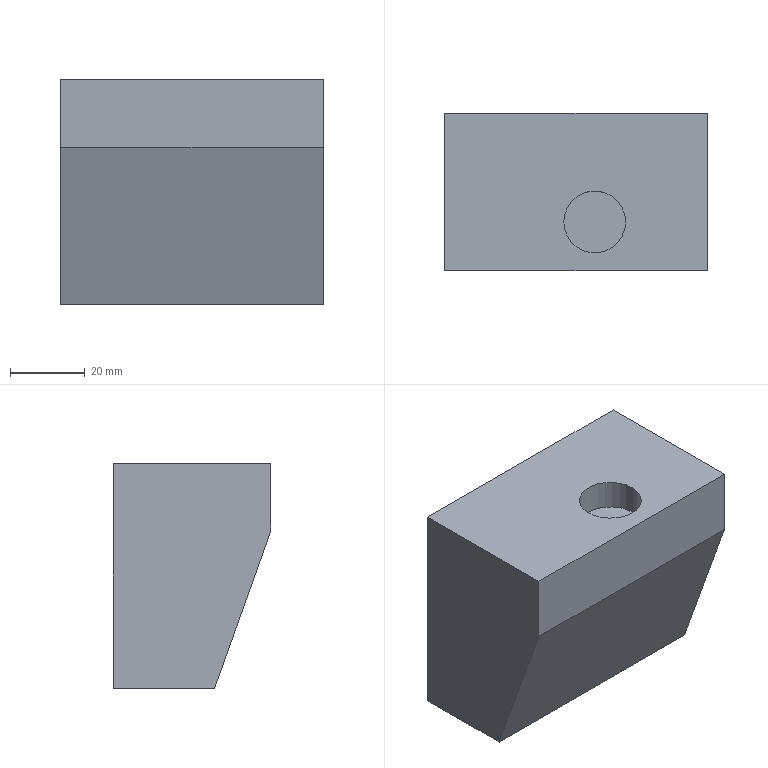Part | SolidWorks | features ICE 2, Extrusion 1 | 1 solid | 10 faces | box 70 x 42 x 60 mm | volume 152639 mm3 | plane 8 | cylinder 2 | commonest cylinder face diameters 16.5 x2
STEP:
#1=CARTESIAN_POINT('',(-8.25,-9.,22.));
#2=VERTEX_POINT('',#1);
#3=CARTESIAN_POINT('',(8.25,-9.,22.));
#4=VERTEX_POINT('',#3);
#5=CARTESIAN_POINT('',(0.,-9.,22.));
#6=DIRECTION('',(0.,0.,1.));
#7=DIRECTION('',(1.,0.,0.));
#8=AXIS2_PLACEMENT_3D('',#5,#6,#7);
#9=CIRCLE('',#8,8.25);
#10=EDGE_CURVE('',#2,#4,#9,.T.);
#11=ORIENTED_EDGE('',*,*,#10,.F.);
#12=CARTESIAN_POINT('',(-8.25,-9.,30.));
#13=VERTEX_POINT('',#12);
#14=CARTESIAN_POINT('',(-8.25,-9.,22.));
#15=DIRECTION('',(0.,0.,1.));
#16=VECTOR('',#15,1000.);
#17=LINE('',#14,#16);
#18=EDGE_CURVE('',#2,#13,#17,.T.);
#19=ORIENTED_EDGE('',*,*,#18,.T.);
#20=CARTESIAN_POINT('',(8.25,-9.,30.));
#21=VERTEX_POINT('',#20);
#22=CARTESIAN_POINT('',(0.,-9.,30.));
#23=DIRECTION('',(0.,0.,1.));
#24=DIRECTION('',(1.,0.,0.));
#25=AXIS2_PLACEMENT_3D('',#22,#23,#24);
#26=CIRCLE('',#25,8.25);
#27=EDGE_CURVE('',#13,#21,#26,.T.);
#28=ORIENTED_EDGE('',*,*,#27,.T.);
#29=CARTESIAN_POINT('',(8.25,-9.,22.));
#30=DIRECTION('',(0.,0.,1.));
#31=VECTOR('',#30,1000.);
#32=LINE('',#29,#31);
#33=EDGE_CURVE('',#4,#21,#32,.T.);
#34=ORIENTED_EDGE('',*,*,#33,.F.);
#35=EDGE_LOOP('',(#11,#19,#28,#34));
#36=FACE_OUTER_BOUND('',#35,.T.);
#37=CARTESIAN_POINT('',(0.,-9.,22.));
#38=DIRECTION('',(0.,0.,1.));
#39=DIRECTION('',(1.,0.,0.));
#40=AXIS2_PLACEMENT_3D('',#37,#38,#39);
#41=CYLINDRICAL_SURFACE('',#40,8.25);
#42=ADVANCED_FACE('',(#36),#41,.F.);
#43=CARTESIAN_POINT('',(30.,20.,30.));
#44=VERTEX_POINT('',#43);
#45=CARTESIAN_POINT('',(30.,-22.,30.));
#46=VERTEX_POINT('',#45);
#47=CARTESIAN_POINT('',(30.,20.,30.));
#48=DIRECTION('',(0.,-1.,0.));
#49=VECTOR('',#48,1000.);
#50=LINE('',#47,#49);
#51=EDGE_CURVE('',#44,#46,#50,.T.);
#52=ORIENTED_EDGE('',*,*,#51,.T.);
#53=CARTESIAN_POINT('',(30.,-22.,12.));
#54=VERTEX_POINT('',#53);
#55=CARTESIAN_POINT('',(30.,-22.,12.));
#56=DIRECTION('',(0.,0.,-1.));
#57=VECTOR('',#56,1000.);
#58=LINE('',#55,#57);
#59=EDGE_CURVE('',#46,#54,#58,.T.);
#60=ORIENTED_EDGE('',*,*,#59,.T.);
#61=CARTESIAN_POINT('',(30.,-7.,-30.));
#62=VERTEX_POINT('',#61);
#63=CARTESIAN_POINT('',(30.,-7.,-30.));
#64=DIRECTION('',(0.,0.3363,-0.9417));
#65=VECTOR('',#64,1000.);
#66=LINE('',#63,#65);
#67=EDGE_CURVE('',#54,#62,#66,.T.);
#68=ORIENTED_EDGE('',*,*,#67,.T.);
#69=CARTESIAN_POINT('',(30.,20.,-30.));
#70=VERTEX_POINT('',#69);
#71=CARTESIAN_POINT('',(30.,20.,-30.));
#72=DIRECTION('',(0.,-1.,0.));
#73=VECTOR('',#72,1000.);
#74=LINE('',#71,#73);
#75=EDGE_CURVE('',#70,#62,#74,.T.);
#76=ORIENTED_EDGE('',*,*,#75,.F.);
#77=CARTESIAN_POINT('',(30.,20.,-30.));
#78=DIRECTION('',(0.,0.,-1.));
#79=VECTOR('',#78,1000.);
#80=LINE('',#77,#79);
#81=EDGE_CURVE('',#44,#70,#80,.T.);
#82=ORIENTED_EDGE('',*,*,#81,.F.);
#83=EDGE_LOOP('',(#52,#60,#68,#76,#82));
#84=FACE_OUTER_BOUND('',#83,.T.);
#85=CARTESIAN_POINT('',(30.,20.,-30.));
#86=DIRECTION('',(-1.,0.,0.));
#87=DIRECTION('',(0.,0.,1.));
#88=AXIS2_PLACEMENT_3D('',#85,#86,#87);
#89=PLANE('',#88);
#90=ADVANCED_FACE('',(#84),#89,.F.);
#91=ORIENTED_EDGE('',*,*,#75,.T.);
#92=CARTESIAN_POINT('',(-40.,-7.,-30.));
#93=VERTEX_POINT('',#92);
#94=CARTESIAN_POINT('',(-40.,-7.,-30.));
#95=DIRECTION('',(1.,0.,0.));
#96=VECTOR('',#95,1000.);
#97=LINE('',#94,#96);
#98=EDGE_CURVE('',#93,#62,#97,.T.);
#99=ORIENTED_EDGE('',*,*,#98,.F.);
#100=CARTESIAN_POINT('',(-40.,20.,-30.));
#101=VERTEX_POINT('',#100);
#102=CARTESIAN_POINT('',(-40.,0.,-30.));
#103=DIRECTION('',(0.,1.,0.));
#104=VECTOR('',#103,1000.);
#105=LINE('',#102,#104);
#106=EDGE_CURVE('',#93,#101,#105,.T.);
#107=ORIENTED_EDGE('',*,*,#106,.T.);
#108=CARTESIAN_POINT('',(-30.,20.,-30.));
#109=DIRECTION('',(-1.,0.,0.));
#110=VECTOR('',#109,1000.);
#111=LINE('',#108,#110);
#112=EDGE_CURVE('',#70,#101,#111,.T.);
#113=ORIENTED_EDGE('',*,*,#112,.F.);
#114=EDGE_LOOP('',(#91,#99,#107,#113));
#115=FACE_OUTER_BOUND('',#114,.T.);
#116=CARTESIAN_POINT('',(-30.,20.,-30.));
#117=DIRECTION('',(0.,0.,1.));
#118=DIRECTION('',(1.,0.,0.));
#119=AXIS2_PLACEMENT_3D('',#116,#117,#118);
#120=PLANE('',#119);
#121=ADVANCED_FACE('',(#115),#120,.F.);
#122=CARTESIAN_POINT('',(0.,-9.,30.));
#123=DIRECTION('',(0.,0.,1.));
#124=DIRECTION('',(1.,0.,0.));
#125=AXIS2_PLACEMENT_3D('',#122,#123,#124);
#126=CIRCLE('',#125,8.25);
#127=EDGE_CURVE('',#21,#13,#126,.T.);
#128=ORIENTED_EDGE('',*,*,#127,.F.);
#129=ORIENTED_EDGE('',*,*,#27,.F.);
#130=EDGE_LOOP('',(#128,#129));
#131=FACE_BOUND('',#130,.T.);
#132=CARTESIAN_POINT('',(-40.,20.,30.));
#133=VERTEX_POINT('',#132);
#134=CARTESIAN_POINT('',(-30.,20.,30.));
#135=DIRECTION('',(1.,0.,0.));
#136=VECTOR('',#135,1000.);
#137=LINE('',#134,#136);
#138=EDGE_CURVE('',#133,#44,#137,.T.);
#139=ORIENTED_EDGE('',*,*,#138,.F.);
#140=CARTESIAN_POINT('',(-40.,-22.,30.));
#141=VERTEX_POINT('',#140);
#142=CARTESIAN_POINT('',(-40.,-22.,30.));
#143=DIRECTION('',(0.,-1.,0.));
#144=VECTOR('',#143,1000.);
#145=LINE('',#142,#144);
#146=EDGE_CURVE('',#133,#141,#145,.T.);
#147=ORIENTED_EDGE('',*,*,#146,.T.);
#148=CARTESIAN_POINT('',(-40.,-22.,30.));
#149=DIRECTION('',(1.,0.,0.));
#150=VECTOR('',#149,1000.);
#151=LINE('',#148,#150);
#152=EDGE_CURVE('',#141,#46,#151,.T.);
#153=ORIENTED_EDGE('',*,*,#152,.T.);
#154=ORIENTED_EDGE('',*,*,#51,.F.);
#155=EDGE_LOOP('',(#139,#147,#153,#154));
#156=FACE_OUTER_BOUND('',#155,.T.);
#157=CARTESIAN_POINT('',(-30.,20.,30.));
#158=DIRECTION('',(0.,0.,-1.));
#159=DIRECTION('',(-1.,0.,0.));
#160=AXIS2_PLACEMENT_3D('',#157,#158,#159);
#161=PLANE('',#160);
#162=ADVANCED_FACE('',(#131,#156),#161,.F.);
#163=ORIENTED_EDGE('',*,*,#81,.T.);
#164=ORIENTED_EDGE('',*,*,#112,.T.);
#165=CARTESIAN_POINT('',(-40.,20.,30.));
#166=DIRECTION('',(0.,0.,1.));
#167=VECTOR('',#166,1000.);
#168=LINE('',#165,#167);
#169=EDGE_CURVE('',#101,#133,#168,.T.);
#170=ORIENTED_EDGE('',*,*,#169,.T.);
#171=ORIENTED_EDGE('',*,*,#138,.T.);
#172=EDGE_LOOP('',(#163,#164,#170,#171));
#173=FACE_OUTER_BOUND('',#172,.T.);
#174=CARTESIAN_POINT('',(0.,20.,0.));
#175=DIRECTION('',(0.,1.,0.));
#176=DIRECTION('',(0.,0.,1.));
#177=AXIS2_PLACEMENT_3D('',#174,#175,#176);
#178=PLANE('',#177);
#179=ADVANCED_FACE('',(#173),#178,.T.);
#180=ORIENTED_EDGE('',*,*,#67,.F.);
#181=CARTESIAN_POINT('',(-40.,-22.,12.));
#182=VERTEX_POINT('',#181);
#183=CARTESIAN_POINT('',(-40.,-22.,12.));
#184=DIRECTION('',(1.,0.,0.));
#185=VECTOR('',#184,1000.);
#186=LINE('',#183,#185);
#187=EDGE_CURVE('',#182,#54,#186,.T.);
#188=ORIENTED_EDGE('',*,*,#187,.F.);
#189=CARTESIAN_POINT('',(-40.,-7.,-30.));
#190=DIRECTION('',(0.,0.3363,-0.9417));
#191=VECTOR('',#190,1000.);
#192=LINE('',#189,#191);
#193=EDGE_CURVE('',#182,#93,#192,.T.);
#194=ORIENTED_EDGE('',*,*,#193,.T.);
#195=ORIENTED_EDGE('',*,*,#98,.T.);
#196=EDGE_LOOP('',(#180,#188,#194,#195));
#197=FACE_OUTER_BOUND('',#196,.T.);
#198=CARTESIAN_POINT('',(-40.,-7.,-30.));
#199=DIRECTION('',(0.,-0.9417,-0.3363));
#200=DIRECTION('',(0.,0.3363,-0.9417));
#201=AXIS2_PLACEMENT_3D('',#198,#199,#200);
#202=PLANE('',#201);
#203=ADVANCED_FACE('',(#197),#202,.T.);
#204=ORIENTED_EDGE('',*,*,#59,.F.);
#205=ORIENTED_EDGE('',*,*,#152,.F.);
#206=CARTESIAN_POINT('',(-40.,-22.,12.));
#207=DIRECTION('',(0.,0.,-1.));
#208=VECTOR('',#207,1000.);
#209=LINE('',#206,#208);
#210=EDGE_CURVE('',#141,#182,#209,.T.);
#211=ORIENTED_EDGE('',*,*,#210,.T.);
#212=ORIENTED_EDGE('',*,*,#187,.T.);
#213=EDGE_LOOP('',(#204,#205,#211,#212));
#214=FACE_OUTER_BOUND('',#213,.T.);
#215=CARTESIAN_POINT('',(-40.,-22.,12.));
#216=DIRECTION('',(0.,-1.,0.));
#217=DIRECTION('',(0.,0.,-1.));
#218=AXIS2_PLACEMENT_3D('',#215,#216,#217);
#219=PLANE('',#218);
#220=ADVANCED_FACE('',(#214),#219,.T.);
#221=ORIENTED_EDGE('',*,*,#169,.F.);
#222=ORIENTED_EDGE('',*,*,#106,.F.);
#223=ORIENTED_EDGE('',*,*,#193,.F.);
#224=ORIENTED_EDGE('',*,*,#210,.F.);
#225=ORIENTED_EDGE('',*,*,#146,.F.);
#226=EDGE_LOOP('',(#221,#222,#223,#224,#225));
#227=FACE_OUTER_BOUND('',#226,.T.);
#228=CARTESIAN_POINT('',(-40.,0.,0.));
#229=DIRECTION('',(-1.,0.,0.));
#230=DIRECTION('',(0.,0.,1.));
#231=AXIS2_PLACEMENT_3D('',#228,#229,#230);
#232=PLANE('',#231);
#233=ADVANCED_FACE('',(#227),#232,.T.);
#234=ORIENTED_EDGE('',*,*,#18,.F.);
#235=CARTESIAN_POINT('',(0.,-9.,22.));
#236=DIRECTION('',(0.,0.,1.));
#237=DIRECTION('',(1.,0.,0.));
#238=AXIS2_PLACEMENT_3D('',#235,#236,#237);
#239=CIRCLE('',#238,8.25);
#240=EDGE_CURVE('',#4,#2,#239,.T.);
#241=ORIENTED_EDGE('',*,*,#240,.F.);
#242=ORIENTED_EDGE('',*,*,#33,.T.);
#243=ORIENTED_EDGE('',*,*,#127,.T.);
#244=EDGE_LOOP('',(#234,#241,#242,#243));
#245=FACE_OUTER_BOUND('',#244,.T.);
#246=CARTESIAN_POINT('',(0.,-9.,22.));
#247=DIRECTION('',(0.,0.,1.));
#248=DIRECTION('',(1.,0.,0.));
#249=AXIS2_PLACEMENT_3D('',#246,#247,#248);
#250=CYLINDRICAL_SURFACE('',#249,8.25);
#251=ADVANCED_FACE('',(#245),#250,.F.);
#252=ORIENTED_EDGE('',*,*,#240,.T.);
#253=ORIENTED_EDGE('',*,*,#10,.T.);
#254=EDGE_LOOP('',(#252,#253));
#255=FACE_OUTER_BOUND('',#254,.T.);
#256=CARTESIAN_POINT('',(0.,-9.,22.));
#257=DIRECTION('',(0.,0.,1.));
#258=DIRECTION('',(1.,0.,0.));
#259=AXIS2_PLACEMENT_3D('',#256,#257,#258);
#260=PLANE('',#259);
#261=ADVANCED_FACE('',(#255),#260,.T.);
#262=CLOSED_SHELL('',(#42,#90,#121,#162,#179,#203,#220,#233,#251,#261));
#263=MANIFOLD_SOLID_BREP('',#262);
#264=CARTESIAN_POINT('',(0.,0.,0.));
#265=DIRECTION('',(0.,0.,1.));
#266=DIRECTION('',(1.,0.,0.));
#267=AXIS2_PLACEMENT_3D('',#264,#265,#266);
#268=(LENGTH_UNIT()NAMED_UNIT(*)SI_UNIT(.MILLI.,.METRE.));
#269=UNCERTAINTY_MEASURE_WITH_UNIT(LENGTH_MEASURE(0.00001),#268,'','');
#270=(NAMED_UNIT(*)PLANE_ANGLE_UNIT()SI_UNIT($,.RADIAN.));
#271=(NAMED_UNIT(*)SI_UNIT($,.STERADIAN.)SOLID_ANGLE_UNIT());
#272=(GEOMETRIC_REPRESENTATION_CONTEXT(3)GLOBAL_UNCERTAINTY_ASSIGNED_CONTEXT((#269))GLOBAL_UNIT_ASSIGNED_CONTEXT((#268,#270,#271))REPRESENTATION_CONTEXT('',''));
#273=ADVANCED_BREP_SHAPE_REPRESENTATION('',(#263,#267),#272);